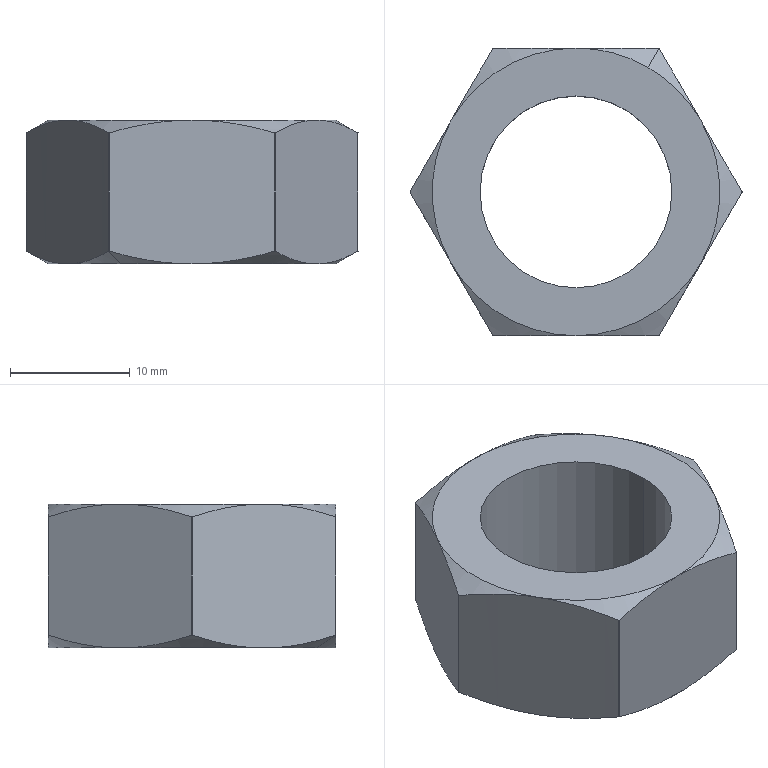Part | STEP file | ~PA16-150_2.stp | 1 solid | 31 faces | box 27.7 x 24 x 12 mm | volume 3543 mm3 | cone 14 | cylinder 9 | plane 8 | commonest cylinder face diameters 27.7 x7 16 x2